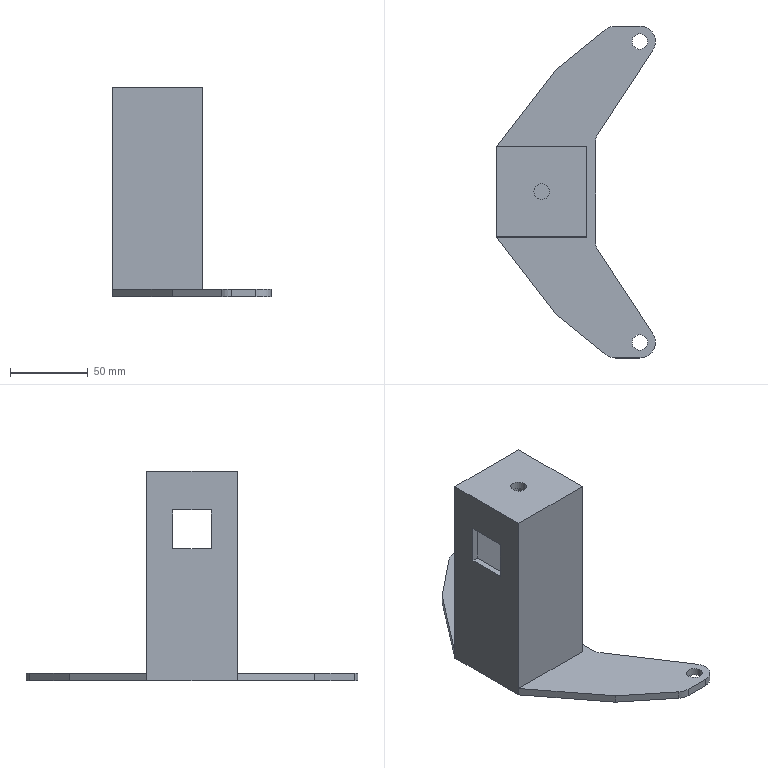Part | STEP file | 1 solid | 44 faces | box 102.124 x 213.51 x 135 mm | volume 177553 mm3 | plane 30 | cylinder 14 | commonest cylinder face diameters 20 x8 10 x6